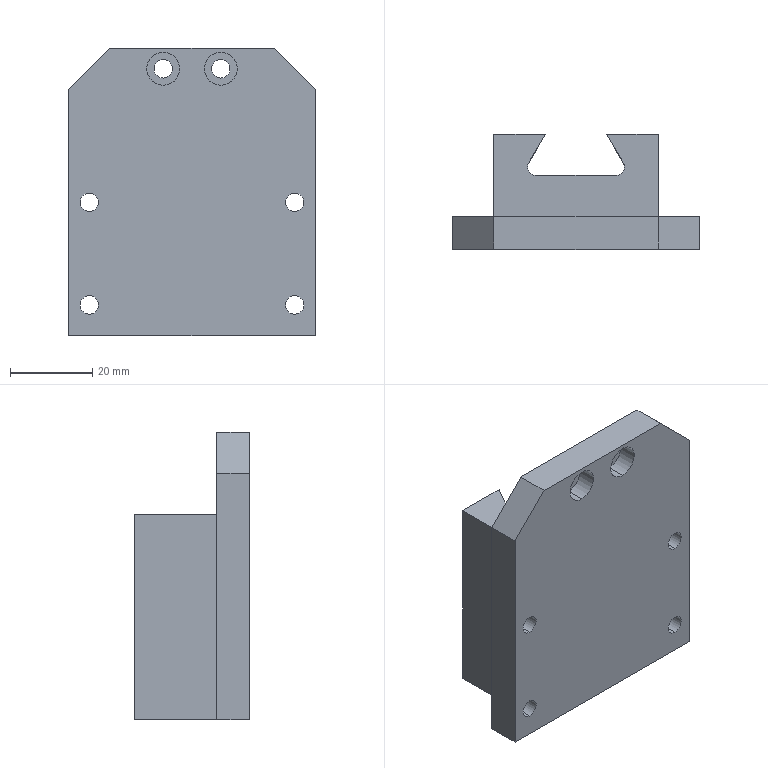Part | SolidWorks | features HoleWzd 4, ICE 2, Chamfer 1, Extrusion 1 | 1 solid | 60 faces | box 60 x 28 x 70 mm | volume 60781 mm3 | cylinder 34 | plane 22 | cone 4 | commonest cylinder face diameters 4.5 x12 8 x12 2.5 x4 4 x4 4.2 x2